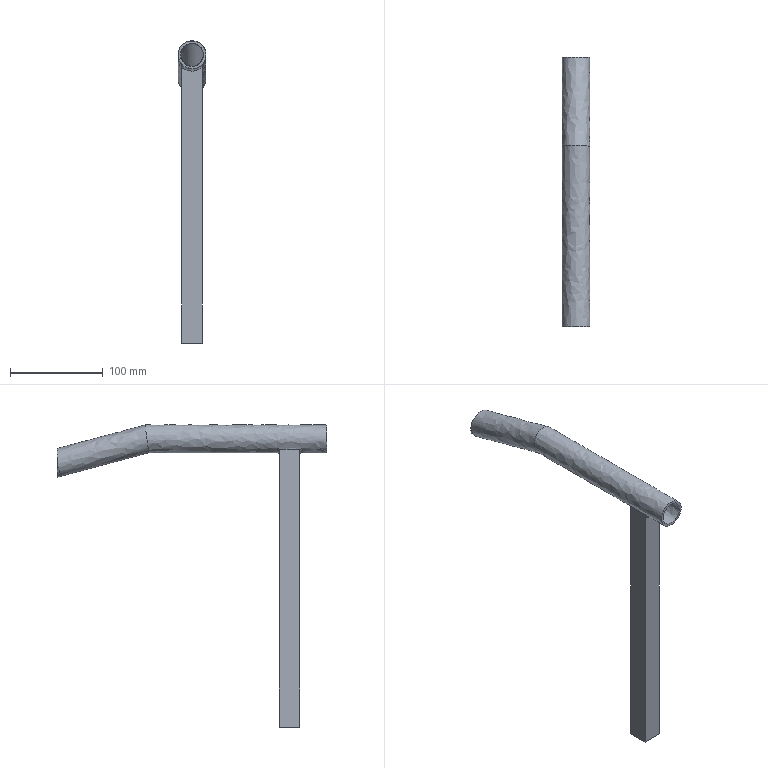Part | NX | features solid 2 | 1 solid | 22 faces | box 30 x 290.001 x 325 mm | volume 121500 mm3 | plane 11 | spline 10 | cylinder 1 | commonest cylinder face diameters 30 x1